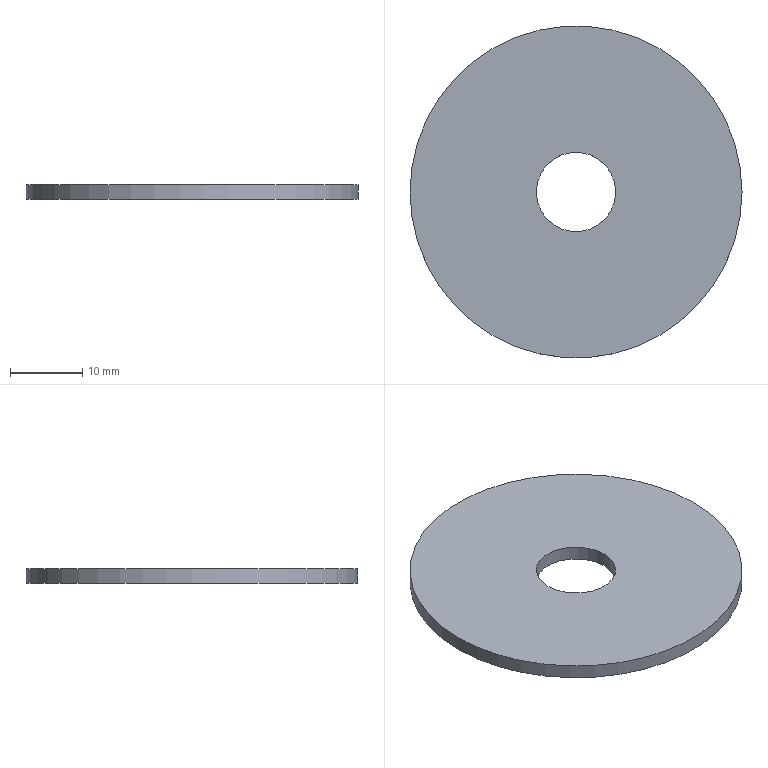Part | NX | features CYLINDER 1, DATUM_CSYS 1, HOLE PACKAGE 1, SIMPLE HOLE 1 | 1 solid | 4 faces | box 46 x 46 x 2 mm | volume 3134 mm3 | plane 2 | cylinder 2 | commonest cylinder face diameters 11 x1 46 x1
STEP:
#1=CARTESIAN_POINT('',(5.5,0.,2.));
#2=VERTEX_POINT('',#1);
#3=CARTESIAN_POINT('',(0.,0.,2.));
#4=DIRECTION('',(0.,0.,1.));
#5=DIRECTION('',(1.,0.,0.));
#6=AXIS2_PLACEMENT_3D('',#3,#4,#5);
#7=CIRCLE('',#6,5.5);
#8=EDGE_CURVE('',#2,#2,#7,.T.);
#9=ORIENTED_EDGE('',*,*,#8,.F.);
#10=EDGE_LOOP('',(#9));
#11=FACE_BOUND('',#10,.T.);
#12=CARTESIAN_POINT('',(-23.,0.,2.));
#13=VERTEX_POINT('',#12);
#14=CARTESIAN_POINT('',(0.,0.,2.));
#15=DIRECTION('',(0.,0.,-1.));
#16=DIRECTION('',(-1.,0.,0.));
#17=AXIS2_PLACEMENT_3D('',#14,#15,#16);
#18=CIRCLE('',#17,23.);
#19=EDGE_CURVE('',#13,#13,#18,.T.);
#20=ORIENTED_EDGE('',*,*,#19,.F.);
#21=EDGE_LOOP('',(#20));
#22=FACE_BOUND('',#21,.T.);
#23=CARTESIAN_POINT('',(0.,0.,2.));
#24=DIRECTION('',(0.,0.,1.));
#25=DIRECTION('',(1.,0.,0.));
#26=AXIS2_PLACEMENT_3D('',#23,#24,#25);
#27=PLANE('',#26);
#28=ADVANCED_FACE('',(#11,#22),#27,.T.);
#29=CARTESIAN_POINT('',(5.5,0.,0.));
#30=VERTEX_POINT('',#29);
#31=CARTESIAN_POINT('',(0.,0.,0.));
#32=DIRECTION('',(0.,0.,1.));
#33=DIRECTION('',(1.,0.,0.));
#34=AXIS2_PLACEMENT_3D('',#31,#32,#33);
#35=CIRCLE('',#34,5.5);
#36=EDGE_CURVE('',#30,#30,#35,.T.);
#37=ORIENTED_EDGE('',*,*,#36,.T.);
#38=EDGE_LOOP('',(#37));
#39=FACE_BOUND('',#38,.T.);
#40=CARTESIAN_POINT('',(23.,0.,0.));
#41=VERTEX_POINT('',#40);
#42=CARTESIAN_POINT('',(0.,0.,0.));
#43=DIRECTION('',(0.,0.,1.));
#44=DIRECTION('',(1.,0.,0.));
#45=AXIS2_PLACEMENT_3D('',#42,#43,#44);
#46=CIRCLE('',#45,23.);
#47=EDGE_CURVE('',#41,#41,#46,.T.);
#48=ORIENTED_EDGE('',*,*,#47,.F.);
#49=EDGE_LOOP('',(#48));
#50=FACE_BOUND('',#49,.T.);
#51=CARTESIAN_POINT('',(0.,0.,0.));
#52=DIRECTION('',(0.,0.,-1.));
#53=DIRECTION('',(-1.,0.,0.));
#54=AXIS2_PLACEMENT_3D('',#51,#52,#53);
#55=PLANE('',#54);
#56=ADVANCED_FACE('',(#39,#50),#55,.T.);
#57=ORIENTED_EDGE('',*,*,#19,.T.);
#58=EDGE_LOOP('',(#57));
#59=FACE_BOUND('',#58,.T.);
#60=ORIENTED_EDGE('',*,*,#47,.T.);
#61=EDGE_LOOP('',(#60));
#62=FACE_BOUND('',#61,.T.);
#63=CARTESIAN_POINT('',(0.,0.,0.));
#64=DIRECTION('',(0.,0.,1.));
#65=DIRECTION('',(1.,0.,0.));
#66=AXIS2_PLACEMENT_3D('',#63,#64,#65);
#67=CYLINDRICAL_SURFACE('',#66,23.);
#68=ADVANCED_FACE('',(#59,#62),#67,.T.);
#69=ORIENTED_EDGE('',*,*,#8,.T.);
#70=EDGE_LOOP('',(#69));
#71=FACE_BOUND('',#70,.T.);
#72=ORIENTED_EDGE('',*,*,#36,.F.);
#73=EDGE_LOOP('',(#72));
#74=FACE_BOUND('',#73,.T.);
#75=CARTESIAN_POINT('',(0.,0.,0.));
#76=DIRECTION('',(0.,0.,1.));
#77=DIRECTION('',(1.,0.,0.));
#78=AXIS2_PLACEMENT_3D('',#75,#76,#77);
#79=CYLINDRICAL_SURFACE('',#78,5.5);
#80=ADVANCED_FACE('',(#71,#74),#79,.F.);
#81=CLOSED_SHELL('',(#28,#56,#68,#80));
#82=MANIFOLD_SOLID_BREP('',#81);
#83=(LENGTH_UNIT()NAMED_UNIT(*)SI_UNIT(.MILLI.,.METRE.));
#84=UNCERTAINTY_MEASURE_WITH_UNIT(LENGTH_MEASURE(0.00001),#83,'','');
#85=(NAMED_UNIT(*)PLANE_ANGLE_UNIT()SI_UNIT($,.RADIAN.));
#86=(NAMED_UNIT(*)SI_UNIT($,.STERADIAN.)SOLID_ANGLE_UNIT());
#87=(GEOMETRIC_REPRESENTATION_CONTEXT(3)GLOBAL_UNCERTAINTY_ASSIGNED_CONTEXT((#84))GLOBAL_UNIT_ASSIGNED_CONTEXT((#83,#85,#86))REPRESENTATION_CONTEXT('',''));
#88=ADVANCED_BREP_SHAPE_REPRESENTATION('',(#82),#87);